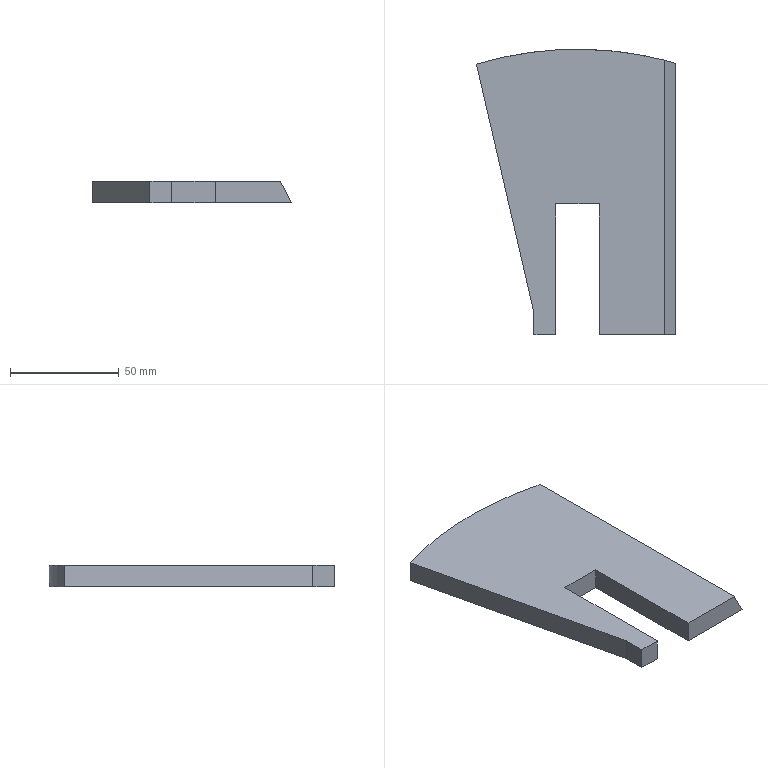Part | SolidWorks | features ICE 2, Extrusion 1 | 1 solid | 11 faces | box 91.361 x 131 x 10 mm | volume 84811 mm3 | plane 10 | cylinder 1 | commonest cylinder face diameters 322 x1
STEP:
#1=CARTESIAN_POINT('',(-20.,30.,-5.));
#2=VERTEX_POINT('',#1);
#3=CARTESIAN_POINT('',(-10.,30.,-5.));
#4=VERTEX_POINT('',#3);
#5=CARTESIAN_POINT('',(0.,30.,-5.));
#6=DIRECTION('',(1.,0.,0.));
#7=VECTOR('',#6,1000.);
#8=LINE('',#5,#7);
#9=EDGE_CURVE('',#2,#4,#8,.T.);
#10=ORIENTED_EDGE('',*,*,#9,.T.);
#11=CARTESIAN_POINT('',(-10.,30.,5.));
#12=VERTEX_POINT('',#11);
#13=CARTESIAN_POINT('',(-10.,30.,5.));
#14=DIRECTION('',(0.,0.,1.));
#15=VECTOR('',#14,1000.);
#16=LINE('',#13,#15);
#17=EDGE_CURVE('',#4,#12,#16,.T.);
#18=ORIENTED_EDGE('',*,*,#17,.T.);
#19=CARTESIAN_POINT('',(-20.,30.,5.));
#20=VERTEX_POINT('',#19);
#21=CARTESIAN_POINT('',(-20.,30.,5.));
#22=DIRECTION('',(1.,0.,0.));
#23=VECTOR('',#22,1000.);
#24=LINE('',#21,#23);
#25=EDGE_CURVE('',#20,#12,#24,.T.);
#26=ORIENTED_EDGE('',*,*,#25,.F.);
#27=CARTESIAN_POINT('',(-20.,30.,5.));
#28=DIRECTION('',(0.,0.,-1.));
#29=VECTOR('',#28,1000.);
#30=LINE('',#27,#29);
#31=EDGE_CURVE('',#20,#2,#30,.T.);
#32=ORIENTED_EDGE('',*,*,#31,.T.);
#33=EDGE_LOOP('',(#10,#18,#26,#32));
#34=FACE_OUTER_BOUND('',#33,.T.);
#35=CARTESIAN_POINT('',(0.,30.,5.));
#36=DIRECTION('',(0.,1.,0.));
#37=DIRECTION('',(0.,0.,1.));
#38=AXIS2_PLACEMENT_3D('',#35,#36,#37);
#39=PLANE('',#38);
#40=ADVANCED_FACE('',(#34),#39,.F.);
#41=CARTESIAN_POINT('',(39.905,155.976,5.));
#42=VERTEX_POINT('',#41);
#43=CARTESIAN_POINT('',(-46.361,154.181,5.));
#44=VERTEX_POINT('',#43);
#45=CARTESIAN_POINT('',(0.,0.,5.));
#46=DIRECTION('',(0.,0.,1.));
#47=DIRECTION('',(1.,0.,0.));
#48=AXIS2_PLACEMENT_3D('',#45,#46,#47);
#49=CIRCLE('',#48,161.);
#50=EDGE_CURVE('',#42,#44,#49,.T.);
#51=ORIENTED_EDGE('',*,*,#50,.F.);
#52=CARTESIAN_POINT('',(45.,154.583,-5.));
#53=VERTEX_POINT('',#52);
#54=CARTESIAN_POINT('',(39.905,155.976,5.));
#55=CARTESIAN_POINT('',(41.611,155.54,1.652));
#56=CARTESIAN_POINT('',(43.309,155.075,-1.682));
#57=CARTESIAN_POINT('',(45.,154.583,-5.));
#58=(BOUNDED_CURVE()B_SPLINE_CURVE(3,(#54,#55,#56,#57),.UNSPECIFIED.,.F.,.F.)B_SPLINE_CURVE_WITH_KNOTS((4,4),(4.963,4.996),.UNSPECIFIED.)CURVE()GEOMETRIC_REPRESENTATION_ITEM()RATIONAL_B_SPLINE_CURVE((1.,0.9999,0.9999,1.))REPRESENTATION_ITEM(''));
#59=EDGE_CURVE('',#42,#53,#58,.T.);
#60=ORIENTED_EDGE('',*,*,#59,.T.);
#61=CARTESIAN_POINT('',(-46.361,154.181,-5.));
#62=VERTEX_POINT('',#61);
#63=CARTESIAN_POINT('',(0.,0.,-5.));
#64=DIRECTION('',(0.,0.,1.));
#65=DIRECTION('',(1.,0.,0.));
#66=AXIS2_PLACEMENT_3D('',#63,#64,#65);
#67=CIRCLE('',#66,161.);
#68=EDGE_CURVE('',#53,#62,#67,.T.);
#69=ORIENTED_EDGE('',*,*,#68,.T.);
#70=CARTESIAN_POINT('',(-46.361,154.181,5.));
#71=DIRECTION('',(0.,0.,-1.));
#72=VECTOR('',#71,1000.);
#73=LINE('',#70,#72);
#74=EDGE_CURVE('',#44,#62,#73,.T.);
#75=ORIENTED_EDGE('',*,*,#74,.F.);
#76=EDGE_LOOP('',(#51,#60,#69,#75));
#77=FACE_OUTER_BOUND('',#76,.T.);
#78=CARTESIAN_POINT('',(0.,0.,5.));
#79=DIRECTION('',(0.,0.,-1.));
#80=DIRECTION('',(-1.,0.,0.));
#81=AXIS2_PLACEMENT_3D('',#78,#79,#80);
#82=CYLINDRICAL_SURFACE('',#81,161.);
#83=ADVANCED_FACE('',(#77),#82,.T.);
#84=CARTESIAN_POINT('',(-20.,40.,-5.));
#85=VERTEX_POINT('',#84);
#86=CARTESIAN_POINT('',(-46.361,154.181,-5.));
#87=DIRECTION('',(0.225,-0.9744,0.));
#88=VECTOR('',#87,1000.);
#89=LINE('',#86,#88);
#90=EDGE_CURVE('',#62,#85,#89,.T.);
#91=ORIENTED_EDGE('',*,*,#90,.T.);
#92=CARTESIAN_POINT('',(-20.,40.,5.));
#93=VERTEX_POINT('',#92);
#94=CARTESIAN_POINT('',(-20.,40.,5.));
#95=DIRECTION('',(0.,0.,-1.));
#96=VECTOR('',#95,1000.);
#97=LINE('',#94,#96);
#98=EDGE_CURVE('',#93,#85,#97,.T.);
#99=ORIENTED_EDGE('',*,*,#98,.F.);
#100=CARTESIAN_POINT('',(-46.361,154.181,5.));
#101=DIRECTION('',(0.225,-0.9744,0.));
#102=VECTOR('',#101,1000.);
#103=LINE('',#100,#102);
#104=EDGE_CURVE('',#44,#93,#103,.T.);
#105=ORIENTED_EDGE('',*,*,#104,.F.);
#106=ORIENTED_EDGE('',*,*,#74,.T.);
#107=EDGE_LOOP('',(#91,#99,#105,#106));
#108=FACE_OUTER_BOUND('',#107,.T.);
#109=CARTESIAN_POINT('',(-46.361,154.181,5.));
#110=DIRECTION('',(0.9744,0.225,0.));
#111=DIRECTION('',(-0.225,0.9744,0.));
#112=AXIS2_PLACEMENT_3D('',#109,#110,#111);
#113=PLANE('',#112);
#114=ADVANCED_FACE('',(#108),#113,.F.);
#115=CARTESIAN_POINT('',(-20.,40.,-5.));
#116=DIRECTION('',(0.,-1.,0.));
#117=VECTOR('',#116,1000.);
#118=LINE('',#115,#117);
#119=EDGE_CURVE('',#85,#2,#118,.T.);
#120=ORIENTED_EDGE('',*,*,#119,.T.);
#121=ORIENTED_EDGE('',*,*,#31,.F.);
#122=CARTESIAN_POINT('',(-20.,40.,5.));
#123=DIRECTION('',(0.,-1.,0.));
#124=VECTOR('',#123,1000.);
#125=LINE('',#122,#124);
#126=EDGE_CURVE('',#93,#20,#125,.T.);
#127=ORIENTED_EDGE('',*,*,#126,.F.);
#128=ORIENTED_EDGE('',*,*,#98,.T.);
#129=EDGE_LOOP('',(#120,#121,#127,#128));
#130=FACE_OUTER_BOUND('',#129,.T.);
#131=CARTESIAN_POINT('',(-20.,40.,5.));
#132=DIRECTION('',(1.,0.,0.));
#133=DIRECTION('',(0.,1.,0.));
#134=AXIS2_PLACEMENT_3D('',#131,#132,#133);
#135=PLANE('',#134);
#136=ADVANCED_FACE('',(#130),#135,.F.);
#137=CARTESIAN_POINT('',(10.,30.,-5.));
#138=VERTEX_POINT('',#137);
#139=CARTESIAN_POINT('',(45.,30.,-5.));
#140=VERTEX_POINT('',#139);
#141=CARTESIAN_POINT('',(0.,30.,-5.));
#142=DIRECTION('',(1.,0.,0.));
#143=VECTOR('',#142,1000.);
#144=LINE('',#141,#143);
#145=EDGE_CURVE('',#138,#140,#144,.T.);
#146=ORIENTED_EDGE('',*,*,#145,.T.);
#147=CARTESIAN_POINT('',(39.905,30.,5.));
#148=VERTEX_POINT('',#147);
#149=CARTESIAN_POINT('',(45.,30.,-5.));
#150=DIRECTION('',(0.454,0.,-0.891));
#151=VECTOR('',#150,1000.);
#152=LINE('',#149,#151);
#153=EDGE_CURVE('',#148,#140,#152,.T.);
#154=ORIENTED_EDGE('',*,*,#153,.F.);
#155=CARTESIAN_POINT('',(10.,30.,5.));
#156=VERTEX_POINT('',#155);
#157=CARTESIAN_POINT('',(-20.,30.,5.));
#158=DIRECTION('',(1.,0.,0.));
#159=VECTOR('',#158,1000.);
#160=LINE('',#157,#159);
#161=EDGE_CURVE('',#156,#148,#160,.T.);
#162=ORIENTED_EDGE('',*,*,#161,.F.);
#163=CARTESIAN_POINT('',(10.,30.,5.));
#164=DIRECTION('',(0.,0.,-1.));
#165=VECTOR('',#164,1000.);
#166=LINE('',#163,#165);
#167=EDGE_CURVE('',#156,#138,#166,.T.);
#168=ORIENTED_EDGE('',*,*,#167,.T.);
#169=EDGE_LOOP('',(#146,#154,#162,#168));
#170=FACE_OUTER_BOUND('',#169,.T.);
#171=CARTESIAN_POINT('',(0.,30.,5.));
#172=DIRECTION('',(0.,1.,0.));
#173=DIRECTION('',(0.,0.,1.));
#174=AXIS2_PLACEMENT_3D('',#171,#172,#173);
#175=PLANE('',#174);
#176=ADVANCED_FACE('',(#170),#175,.F.);
#177=CARTESIAN_POINT('',(39.905,161.,5.));
#178=DIRECTION('',(0.,-1.,0.));
#179=VECTOR('',#178,1000.);
#180=LINE('',#177,#179);
#181=EDGE_CURVE('',#42,#148,#180,.T.);
#182=ORIENTED_EDGE('',*,*,#181,.F.);
#183=ORIENTED_EDGE('',*,*,#50,.T.);
#184=ORIENTED_EDGE('',*,*,#104,.T.);
#185=ORIENTED_EDGE('',*,*,#126,.T.);
#186=ORIENTED_EDGE('',*,*,#25,.T.);
#187=CARTESIAN_POINT('',(-10.,90.,5.));
#188=VERTEX_POINT('',#187);
#189=CARTESIAN_POINT('',(-10.,-30.,5.));
#190=DIRECTION('',(0.,-1.,0.));
#191=VECTOR('',#190,1000.);
#192=LINE('',#189,#191);
#193=EDGE_CURVE('',#188,#12,#192,.T.);
#194=ORIENTED_EDGE('',*,*,#193,.F.);
#195=CARTESIAN_POINT('',(10.,90.,5.));
#196=VERTEX_POINT('',#195);
#197=CARTESIAN_POINT('',(10.,90.,5.));
#198=DIRECTION('',(-1.,0.,0.));
#199=VECTOR('',#198,1000.);
#200=LINE('',#197,#199);
#201=EDGE_CURVE('',#196,#188,#200,.T.);
#202=ORIENTED_EDGE('',*,*,#201,.F.);
#203=CARTESIAN_POINT('',(10.,-30.,5.));
#204=DIRECTION('',(0.,1.,0.));
#205=VECTOR('',#204,1000.);
#206=LINE('',#203,#205);
#207=EDGE_CURVE('',#156,#196,#206,.T.);
#208=ORIENTED_EDGE('',*,*,#207,.F.);
#209=ORIENTED_EDGE('',*,*,#161,.T.);
#210=EDGE_LOOP('',(#182,#183,#184,#185,#186,#194,#202,#208,#209));
#211=FACE_OUTER_BOUND('',#210,.T.);
#212=CARTESIAN_POINT('',(0.,0.,5.));
#213=DIRECTION('',(0.,0.,1.));
#214=DIRECTION('',(1.,0.,0.));
#215=AXIS2_PLACEMENT_3D('',#212,#213,#214);
#216=PLANE('',#215);
#217=ADVANCED_FACE('',(#211),#216,.T.);
#218=CARTESIAN_POINT('',(10.,90.,-5.));
#219=VERTEX_POINT('',#218);
#220=CARTESIAN_POINT('',(-10.,90.,-5.));
#221=VERTEX_POINT('',#220);
#222=CARTESIAN_POINT('',(10.,90.,-5.));
#223=DIRECTION('',(-1.,0.,0.));
#224=VECTOR('',#223,1000.);
#225=LINE('',#222,#224);
#226=EDGE_CURVE('',#219,#221,#225,.T.);
#227=ORIENTED_EDGE('',*,*,#226,.T.);
#228=CARTESIAN_POINT('',(-10.,-30.,-5.));
#229=DIRECTION('',(0.,-1.,0.));
#230=VECTOR('',#229,1000.);
#231=LINE('',#228,#230);
#232=EDGE_CURVE('',#221,#4,#231,.T.);
#233=ORIENTED_EDGE('',*,*,#232,.T.);
#234=ORIENTED_EDGE('',*,*,#9,.F.);
#235=ORIENTED_EDGE('',*,*,#119,.F.);
#236=ORIENTED_EDGE('',*,*,#90,.F.);
#237=ORIENTED_EDGE('',*,*,#68,.F.);
#238=CARTESIAN_POINT('',(45.,40.,-5.));
#239=DIRECTION('',(0.,1.,0.));
#240=VECTOR('',#239,1000.);
#241=LINE('',#238,#240);
#242=EDGE_CURVE('',#140,#53,#241,.T.);
#243=ORIENTED_EDGE('',*,*,#242,.F.);
#244=ORIENTED_EDGE('',*,*,#145,.F.);
#245=CARTESIAN_POINT('',(10.,0.,-5.));
#246=DIRECTION('',(0.,1.,0.));
#247=VECTOR('',#246,1000.);
#248=LINE('',#245,#247);
#249=EDGE_CURVE('',#138,#219,#248,.T.);
#250=ORIENTED_EDGE('',*,*,#249,.T.);
#251=EDGE_LOOP('',(#227,#233,#234,#235,#236,#237,#243,#244,#250));
#252=FACE_OUTER_BOUND('',#251,.T.);
#253=CARTESIAN_POINT('',(0.,0.,-5.));
#254=DIRECTION('',(0.,0.,1.));
#255=DIRECTION('',(1.,0.,0.));
#256=AXIS2_PLACEMENT_3D('',#253,#254,#255);
#257=PLANE('',#256);
#258=ADVANCED_FACE('',(#252),#257,.F.);
#259=ORIENTED_EDGE('',*,*,#232,.F.);
#260=CARTESIAN_POINT('',(-10.,90.,-5.));
#261=DIRECTION('',(0.,0.,1.));
#262=VECTOR('',#261,1000.);
#263=LINE('',#260,#262);
#264=EDGE_CURVE('',#221,#188,#263,.T.);
#265=ORIENTED_EDGE('',*,*,#264,.T.);
#266=ORIENTED_EDGE('',*,*,#193,.T.);
#267=ORIENTED_EDGE('',*,*,#17,.F.);
#268=EDGE_LOOP('',(#259,#265,#266,#267));
#269=FACE_OUTER_BOUND('',#268,.T.);
#270=CARTESIAN_POINT('',(-10.,-30.,-5.));
#271=DIRECTION('',(-1.,0.,0.));
#272=DIRECTION('',(0.,0.,1.));
#273=AXIS2_PLACEMENT_3D('',#270,#271,#272);
#274=PLANE('',#273);
#275=ADVANCED_FACE('',(#269),#274,.F.);
#276=ORIENTED_EDGE('',*,*,#207,.T.);
#277=CARTESIAN_POINT('',(10.,90.,-5.));
#278=DIRECTION('',(0.,0.,1.));
#279=VECTOR('',#278,1000.);
#280=LINE('',#277,#279);
#281=EDGE_CURVE('',#219,#196,#280,.T.);
#282=ORIENTED_EDGE('',*,*,#281,.F.);
#283=ORIENTED_EDGE('',*,*,#249,.F.);
#284=ORIENTED_EDGE('',*,*,#167,.F.);
#285=EDGE_LOOP('',(#276,#282,#283,#284));
#286=FACE_OUTER_BOUND('',#285,.T.);
#287=CARTESIAN_POINT('',(10.,-30.,-5.));
#288=DIRECTION('',(1.,0.,0.));
#289=DIRECTION('',(0.,0.,-1.));
#290=AXIS2_PLACEMENT_3D('',#287,#288,#289);
#291=PLANE('',#290);
#292=ADVANCED_FACE('',(#286),#291,.F.);
#293=ORIENTED_EDGE('',*,*,#201,.T.);
#294=ORIENTED_EDGE('',*,*,#264,.F.);
#295=ORIENTED_EDGE('',*,*,#226,.F.);
#296=ORIENTED_EDGE('',*,*,#281,.T.);
#297=EDGE_LOOP('',(#293,#294,#295,#296));
#298=FACE_OUTER_BOUND('',#297,.T.);
#299=CARTESIAN_POINT('',(10.,90.,-5.));
#300=DIRECTION('',(0.,1.,0.));
#301=DIRECTION('',(0.,0.,1.));
#302=AXIS2_PLACEMENT_3D('',#299,#300,#301);
#303=PLANE('',#302);
#304=ADVANCED_FACE('',(#298),#303,.F.);
#305=ORIENTED_EDGE('',*,*,#181,.T.);
#306=ORIENTED_EDGE('',*,*,#153,.T.);
#307=ORIENTED_EDGE('',*,*,#242,.T.);
#308=ORIENTED_EDGE('',*,*,#59,.F.);
#309=EDGE_LOOP('',(#305,#306,#307,#308));
#310=FACE_OUTER_BOUND('',#309,.T.);
#311=CARTESIAN_POINT('',(45.,161.,-5.));
#312=DIRECTION('',(-0.891,0.,-0.454));
#313=DIRECTION('',(-0.454,0.,0.891));
#314=AXIS2_PLACEMENT_3D('',#311,#312,#313);
#315=PLANE('',#314);
#316=ADVANCED_FACE('',(#310),#315,.F.);
#317=CLOSED_SHELL('',(#40,#83,#114,#136,#176,#217,#258,#275,#292,#304,#316));
#318=MANIFOLD_SOLID_BREP('',#317);
#319=CARTESIAN_POINT('',(0.,0.,0.));
#320=DIRECTION('',(0.,0.,1.));
#321=DIRECTION('',(1.,0.,0.));
#322=AXIS2_PLACEMENT_3D('',#319,#320,#321);
#323=(LENGTH_UNIT()NAMED_UNIT(*)SI_UNIT(.MILLI.,.METRE.));
#324=UNCERTAINTY_MEASURE_WITH_UNIT(LENGTH_MEASURE(0.00001),#323,'','');
#325=(NAMED_UNIT(*)PLANE_ANGLE_UNIT()SI_UNIT($,.RADIAN.));
#326=(NAMED_UNIT(*)SI_UNIT($,.STERADIAN.)SOLID_ANGLE_UNIT());
#327=(GEOMETRIC_REPRESENTATION_CONTEXT(3)GLOBAL_UNCERTAINTY_ASSIGNED_CONTEXT((#324))GLOBAL_UNIT_ASSIGNED_CONTEXT((#323,#325,#326))REPRESENTATION_CONTEXT('',''));
#328=ADVANCED_BREP_SHAPE_REPRESENTATION('',(#318,#322),#327);